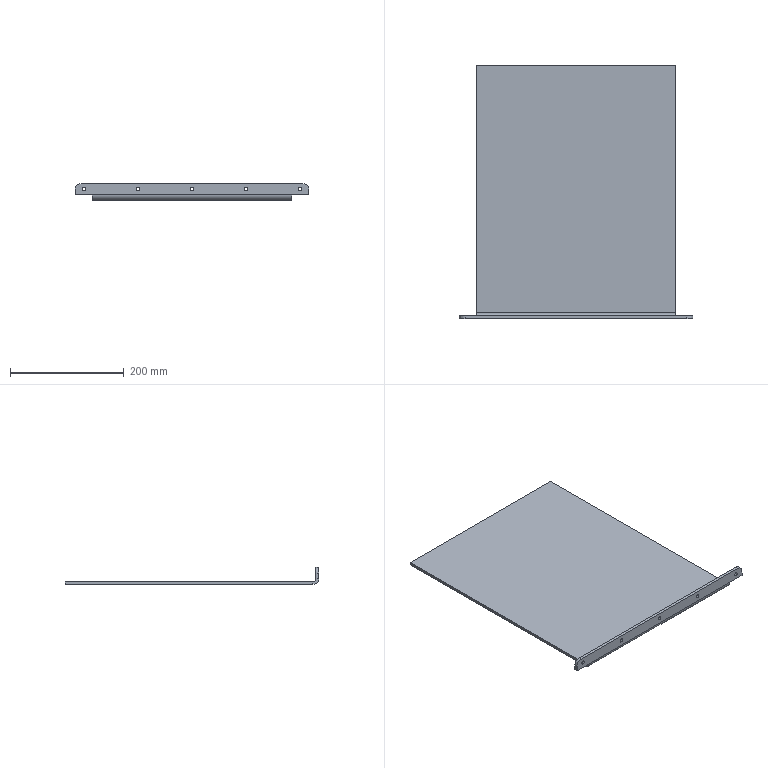Part | SolidWorks | features EdgeFlange 1, Fillet 1, FlatPattern 1, HoleWzd 1, LPattern 1, SMBaseFlange 1, SheetMetal 1 | 1 solid | 38 faces | box 410 x 445 x 30 mm | volume 821945 mm3 | cylinder 14 | plane 14 | cone 10 | commonest cylinder face diameters 6 x10 20 x3 10 x1
STEP:
#1=CARTESIAN_POINT('',(-95.,-222.475,23.));
#2=VERTEX_POINT('',#1);
#3=CARTESIAN_POINT('',(-95.,-222.475,17.));
#4=VERTEX_POINT('',#3);
#5=CARTESIAN_POINT('',(-95.,-222.475,20.));
#6=DIRECTION('',(0.,-1.,0.));
#7=DIRECTION('',(0.,0.,-1.));
#8=AXIS2_PLACEMENT_3D('',#5,#6,#7);
#9=CIRCLE('',#8,3.);
#10=EDGE_CURVE('',#2,#4,#9,.T.);
#11=ORIENTED_EDGE('',*,*,#10,.F.);
#12=CARTESIAN_POINT('',(-95.,-222.5,23.025));
#13=VERTEX_POINT('',#12);
#14=CARTESIAN_POINT('',(-95.,-222.5,23.025));
#15=DIRECTION('',(0.,-0.7071,0.7071));
#16=VECTOR('',#15,1000.);
#17=LINE('',#14,#16);
#18=EDGE_CURVE('',#2,#13,#17,.T.);
#19=ORIENTED_EDGE('',*,*,#18,.T.);
#20=CARTESIAN_POINT('',(-95.,-222.5,16.975));
#21=VERTEX_POINT('',#20);
#22=CARTESIAN_POINT('',(-95.,-222.5,20.));
#23=DIRECTION('',(0.,-1.,0.));
#24=DIRECTION('',(0.,0.,-1.));
#25=AXIS2_PLACEMENT_3D('',#22,#23,#24);
#26=CIRCLE('',#25,3.025);
#27=EDGE_CURVE('',#13,#21,#26,.T.);
#28=ORIENTED_EDGE('',*,*,#27,.T.);
#29=CARTESIAN_POINT('',(-95.,-222.5,16.975));
#30=DIRECTION('',(0.,-0.7071,-0.7071));
#31=VECTOR('',#30,1000.);
#32=LINE('',#29,#31);
#33=EDGE_CURVE('',#4,#21,#32,.T.);
#34=ORIENTED_EDGE('',*,*,#33,.F.);
#35=EDGE_LOOP('',(#11,#19,#28,#34));
#36=FACE_OUTER_BOUND('',#35,.T.);
#37=CARTESIAN_POINT('',(-95.,-222.5,20.));
#38=DIRECTION('',(0.,-1.,0.));
#39=DIRECTION('',(0.,0.,-1.));
#40=AXIS2_PLACEMENT_3D('',#37,#38,#39);
#41=CONICAL_SURFACE('',#40,3.025,0.7854);
#42=ADVANCED_FACE('',(#36),#41,.F.);
#43=CARTESIAN_POINT('',(-95.,-217.5,23.));
#44=VERTEX_POINT('',#43);
#45=CARTESIAN_POINT('',(-95.,-217.5,17.));
#46=VERTEX_POINT('',#45);
#47=CARTESIAN_POINT('',(-95.,-217.5,20.));
#48=DIRECTION('',(0.,-1.,0.));
#49=DIRECTION('',(0.,0.,-1.));
#50=AXIS2_PLACEMENT_3D('',#47,#48,#49);
#51=CIRCLE('',#50,3.);
#52=EDGE_CURVE('',#44,#46,#51,.T.);
#53=ORIENTED_EDGE('',*,*,#52,.F.);
#54=CARTESIAN_POINT('',(-95.,-222.5,23.));
#55=DIRECTION('',(0.,-1.,0.));
#56=VECTOR('',#55,1000.);
#57=LINE('',#54,#56);
#58=EDGE_CURVE('',#44,#2,#57,.T.);
#59=ORIENTED_EDGE('',*,*,#58,.T.);
#60=ORIENTED_EDGE('',*,*,#10,.T.);
#61=CARTESIAN_POINT('',(-95.,-222.5,17.));
#62=DIRECTION('',(0.,-1.,0.));
#63=VECTOR('',#62,1000.);
#64=LINE('',#61,#63);
#65=EDGE_CURVE('',#46,#4,#64,.T.);
#66=ORIENTED_EDGE('',*,*,#65,.F.);
#67=EDGE_LOOP('',(#53,#59,#60,#66));
#68=FACE_OUTER_BOUND('',#67,.T.);
#69=CARTESIAN_POINT('',(-95.,-222.5,20.));
#70=DIRECTION('',(0.,-1.,0.));
#71=DIRECTION('',(0.,0.,-1.));
#72=AXIS2_PLACEMENT_3D('',#69,#70,#71);
#73=CYLINDRICAL_SURFACE('',#72,3.);
#74=ADVANCED_FACE('',(#68),#73,.F.);
#75=CARTESIAN_POINT('',(-190.,-222.475,23.));
#76=VERTEX_POINT('',#75);
#77=CARTESIAN_POINT('',(-190.,-222.475,17.));
#78=VERTEX_POINT('',#77);
#79=CARTESIAN_POINT('',(-190.,-222.475,20.));
#80=DIRECTION('',(0.,-1.,0.));
#81=DIRECTION('',(0.,0.,-1.));
#82=AXIS2_PLACEMENT_3D('',#79,#80,#81);
#83=CIRCLE('',#82,3.);
#84=EDGE_CURVE('',#76,#78,#83,.T.);
#85=ORIENTED_EDGE('',*,*,#84,.F.);
#86=CARTESIAN_POINT('',(-190.,-222.5,23.025));
#87=VERTEX_POINT('',#86);
#88=CARTESIAN_POINT('',(-190.,-222.5,23.025));
#89=DIRECTION('',(0.,-0.7071,0.7071));
#90=VECTOR('',#89,1000.);
#91=LINE('',#88,#90);
#92=EDGE_CURVE('',#76,#87,#91,.T.);
#93=ORIENTED_EDGE('',*,*,#92,.T.);
#94=CARTESIAN_POINT('',(-190.,-222.5,16.975));
#95=VERTEX_POINT('',#94);
#96=CARTESIAN_POINT('',(-190.,-222.5,20.));
#97=DIRECTION('',(0.,-1.,0.));
#98=DIRECTION('',(0.,0.,-1.));
#99=AXIS2_PLACEMENT_3D('',#96,#97,#98);
#100=CIRCLE('',#99,3.025);
#101=EDGE_CURVE('',#87,#95,#100,.T.);
#102=ORIENTED_EDGE('',*,*,#101,.T.);
#103=CARTESIAN_POINT('',(-190.,-222.5,16.975));
#104=DIRECTION('',(0.,-0.7071,-0.7071));
#105=VECTOR('',#104,1000.);
#106=LINE('',#103,#105);
#107=EDGE_CURVE('',#78,#95,#106,.T.);
#108=ORIENTED_EDGE('',*,*,#107,.F.);
#109=EDGE_LOOP('',(#85,#93,#102,#108));
#110=FACE_OUTER_BOUND('',#109,.T.);
#111=CARTESIAN_POINT('',(-190.,-222.5,20.));
#112=DIRECTION('',(0.,-1.,0.));
#113=DIRECTION('',(0.,0.,-1.));
#114=AXIS2_PLACEMENT_3D('',#111,#112,#113);
#115=CONICAL_SURFACE('',#114,3.025,0.7854);
#116=ADVANCED_FACE('',(#110),#115,.F.);
#117=CARTESIAN_POINT('',(-190.,-217.5,23.));
#118=VERTEX_POINT('',#117);
#119=CARTESIAN_POINT('',(-190.,-217.5,17.));
#120=VERTEX_POINT('',#119);
#121=CARTESIAN_POINT('',(-190.,-217.5,20.));
#122=DIRECTION('',(0.,-1.,0.));
#123=DIRECTION('',(0.,0.,-1.));
#124=AXIS2_PLACEMENT_3D('',#121,#122,#123);
#125=CIRCLE('',#124,3.);
#126=EDGE_CURVE('',#118,#120,#125,.T.);
#127=ORIENTED_EDGE('',*,*,#126,.F.);
#128=CARTESIAN_POINT('',(-190.,-222.5,23.));
#129=DIRECTION('',(0.,-1.,0.));
#130=VECTOR('',#129,1000.);
#131=LINE('',#128,#130);
#132=EDGE_CURVE('',#118,#76,#131,.T.);
#133=ORIENTED_EDGE('',*,*,#132,.T.);
#134=ORIENTED_EDGE('',*,*,#84,.T.);
#135=CARTESIAN_POINT('',(-190.,-222.5,17.));
#136=DIRECTION('',(0.,-1.,0.));
#137=VECTOR('',#136,1000.);
#138=LINE('',#135,#137);
#139=EDGE_CURVE('',#120,#78,#138,.T.);
#140=ORIENTED_EDGE('',*,*,#139,.F.);
#141=EDGE_LOOP('',(#127,#133,#134,#140));
#142=FACE_OUTER_BOUND('',#141,.T.);
#143=CARTESIAN_POINT('',(-190.,-222.5,20.));
#144=DIRECTION('',(0.,-1.,0.));
#145=DIRECTION('',(0.,0.,-1.));
#146=AXIS2_PLACEMENT_3D('',#143,#144,#145);
#147=CYLINDRICAL_SURFACE('',#146,3.);
#148=ADVANCED_FACE('',(#142),#147,.F.);
#149=CARTESIAN_POINT('',(0.,-217.5,23.));
#150=VERTEX_POINT('',#149);
#151=CARTESIAN_POINT('',(0.,-217.5,17.));
#152=VERTEX_POINT('',#151);
#153=CARTESIAN_POINT('',(0.,-217.5,20.));
#154=DIRECTION('',(0.,-1.,0.));
#155=DIRECTION('',(0.,0.,-1.));
#156=AXIS2_PLACEMENT_3D('',#153,#154,#155);
#157=CIRCLE('',#156,3.);
#158=EDGE_CURVE('',#150,#152,#157,.T.);
#159=ORIENTED_EDGE('',*,*,#158,.F.);
#160=CARTESIAN_POINT('',(0.,-222.475,23.));
#161=VERTEX_POINT('',#160);
#162=CARTESIAN_POINT('',(0.,-222.5,23.));
#163=DIRECTION('',(0.,-1.,0.));
#164=VECTOR('',#163,1000.);
#165=LINE('',#162,#164);
#166=EDGE_CURVE('',#150,#161,#165,.T.);
#167=ORIENTED_EDGE('',*,*,#166,.T.);
#168=CARTESIAN_POINT('',(0.,-222.475,17.));
#169=VERTEX_POINT('',#168);
#170=CARTESIAN_POINT('',(0.,-222.475,20.));
#171=DIRECTION('',(0.,-1.,0.));
#172=DIRECTION('',(0.,0.,-1.));
#173=AXIS2_PLACEMENT_3D('',#170,#171,#172);
#174=CIRCLE('',#173,3.);
#175=EDGE_CURVE('',#161,#169,#174,.T.);
#176=ORIENTED_EDGE('',*,*,#175,.T.);
#177=CARTESIAN_POINT('',(0.,-222.5,17.));
#178=DIRECTION('',(0.,-1.,0.));
#179=VECTOR('',#178,1000.);
#180=LINE('',#177,#179);
#181=EDGE_CURVE('',#152,#169,#180,.T.);
#182=ORIENTED_EDGE('',*,*,#181,.F.);
#183=EDGE_LOOP('',(#159,#167,#176,#182));
#184=FACE_OUTER_BOUND('',#183,.T.);
#185=CARTESIAN_POINT('',(0.,-222.5,20.));
#186=DIRECTION('',(0.,-1.,0.));
#187=DIRECTION('',(0.,0.,-1.));
#188=AXIS2_PLACEMENT_3D('',#185,#186,#187);
#189=CYLINDRICAL_SURFACE('',#188,3.);
#190=ADVANCED_FACE('',(#184),#189,.F.);
#191=ORIENTED_EDGE('',*,*,#175,.F.);
#192=CARTESIAN_POINT('',(0.,-222.5,23.025));
#193=VERTEX_POINT('',#192);
#194=CARTESIAN_POINT('',(0.,-222.5,23.025));
#195=DIRECTION('',(0.,-0.7071,0.7071));
#196=VECTOR('',#195,1000.);
#197=LINE('',#194,#196);
#198=EDGE_CURVE('',#161,#193,#197,.T.);
#199=ORIENTED_EDGE('',*,*,#198,.T.);
#200=CARTESIAN_POINT('',(0.,-222.5,16.975));
#201=VERTEX_POINT('',#200);
#202=CARTESIAN_POINT('',(0.,-222.5,20.));
#203=DIRECTION('',(0.,-1.,0.));
#204=DIRECTION('',(0.,0.,-1.));
#205=AXIS2_PLACEMENT_3D('',#202,#203,#204);
#206=CIRCLE('',#205,3.025);
#207=EDGE_CURVE('',#193,#201,#206,.T.);
#208=ORIENTED_EDGE('',*,*,#207,.T.);
#209=CARTESIAN_POINT('',(0.,-222.5,16.975));
#210=DIRECTION('',(0.,-0.7071,-0.7071));
#211=VECTOR('',#210,1000.);
#212=LINE('',#209,#211);
#213=EDGE_CURVE('',#169,#201,#212,.T.);
#214=ORIENTED_EDGE('',*,*,#213,.F.);
#215=EDGE_LOOP('',(#191,#199,#208,#214));
#216=FACE_OUTER_BOUND('',#215,.T.);
#217=CARTESIAN_POINT('',(0.,-222.5,20.));
#218=DIRECTION('',(0.,-1.,0.));
#219=DIRECTION('',(0.,0.,-1.));
#220=AXIS2_PLACEMENT_3D('',#217,#218,#219);
#221=CONICAL_SURFACE('',#220,3.025,0.7854);
#222=ADVANCED_FACE('',(#216),#221,.F.);
#223=CARTESIAN_POINT('',(95.,-217.5,23.));
#224=VERTEX_POINT('',#223);
#225=CARTESIAN_POINT('',(95.,-217.5,17.));
#226=VERTEX_POINT('',#225);
#227=CARTESIAN_POINT('',(95.,-217.5,20.));
#228=DIRECTION('',(0.,-1.,0.));
#229=DIRECTION('',(0.,0.,-1.));
#230=AXIS2_PLACEMENT_3D('',#227,#228,#229);
#231=CIRCLE('',#230,3.);
#232=EDGE_CURVE('',#224,#226,#231,.T.);
#233=ORIENTED_EDGE('',*,*,#232,.F.);
#234=CARTESIAN_POINT('',(95.,-222.475,23.));
#235=VERTEX_POINT('',#234);
#236=CARTESIAN_POINT('',(95.,-222.5,23.));
#237=DIRECTION('',(0.,-1.,0.));
#238=VECTOR('',#237,1000.);
#239=LINE('',#236,#238);
#240=EDGE_CURVE('',#224,#235,#239,.T.);
#241=ORIENTED_EDGE('',*,*,#240,.T.);
#242=CARTESIAN_POINT('',(95.,-222.475,17.));
#243=VERTEX_POINT('',#242);
#244=CARTESIAN_POINT('',(95.,-222.475,20.));
#245=DIRECTION('',(0.,-1.,0.));
#246=DIRECTION('',(0.,0.,-1.));
#247=AXIS2_PLACEMENT_3D('',#244,#245,#246);
#248=CIRCLE('',#247,3.);
#249=EDGE_CURVE('',#235,#243,#248,.T.);
#250=ORIENTED_EDGE('',*,*,#249,.T.);
#251=CARTESIAN_POINT('',(95.,-222.5,17.));
#252=DIRECTION('',(0.,-1.,0.));
#253=VECTOR('',#252,1000.);
#254=LINE('',#251,#253);
#255=EDGE_CURVE('',#226,#243,#254,.T.);
#256=ORIENTED_EDGE('',*,*,#255,.F.);
#257=EDGE_LOOP('',(#233,#241,#250,#256));
#258=FACE_OUTER_BOUND('',#257,.T.);
#259=CARTESIAN_POINT('',(95.,-222.5,20.));
#260=DIRECTION('',(0.,-1.,0.));
#261=DIRECTION('',(0.,0.,-1.));
#262=AXIS2_PLACEMENT_3D('',#259,#260,#261);
#263=CYLINDRICAL_SURFACE('',#262,3.);
#264=ADVANCED_FACE('',(#258),#263,.F.);
#265=ORIENTED_EDGE('',*,*,#249,.F.);
#266=CARTESIAN_POINT('',(95.,-222.5,23.025));
#267=VERTEX_POINT('',#266);
#268=CARTESIAN_POINT('',(95.,-222.5,23.025));
#269=DIRECTION('',(0.,-0.7071,0.7071));
#270=VECTOR('',#269,1000.);
#271=LINE('',#268,#270);
#272=EDGE_CURVE('',#235,#267,#271,.T.);
#273=ORIENTED_EDGE('',*,*,#272,.T.);
#274=CARTESIAN_POINT('',(95.,-222.5,16.975));
#275=VERTEX_POINT('',#274);
#276=CARTESIAN_POINT('',(95.,-222.5,20.));
#277=DIRECTION('',(0.,-1.,0.));
#278=DIRECTION('',(0.,0.,-1.));
#279=AXIS2_PLACEMENT_3D('',#276,#277,#278);
#280=CIRCLE('',#279,3.025);
#281=EDGE_CURVE('',#267,#275,#280,.T.);
#282=ORIENTED_EDGE('',*,*,#281,.T.);
#283=CARTESIAN_POINT('',(95.,-222.5,16.975));
#284=DIRECTION('',(0.,-0.7071,-0.7071));
#285=VECTOR('',#284,1000.);
#286=LINE('',#283,#285);
#287=EDGE_CURVE('',#243,#275,#286,.T.);
#288=ORIENTED_EDGE('',*,*,#287,.F.);
#289=EDGE_LOOP('',(#265,#273,#282,#288));
#290=FACE_OUTER_BOUND('',#289,.T.);
#291=CARTESIAN_POINT('',(95.,-222.5,20.));
#292=DIRECTION('',(0.,-1.,0.));
#293=DIRECTION('',(0.,0.,-1.));
#294=AXIS2_PLACEMENT_3D('',#291,#292,#293);
#295=CONICAL_SURFACE('',#294,3.025,0.7854);
#296=ADVANCED_FACE('',(#290),#295,.F.);
#297=CARTESIAN_POINT('',(190.,-217.5,23.));
#298=VERTEX_POINT('',#297);
#299=CARTESIAN_POINT('',(190.,-217.5,17.));
#300=VERTEX_POINT('',#299);
#301=CARTESIAN_POINT('',(190.,-217.5,20.));
#302=DIRECTION('',(0.,-1.,0.));
#303=DIRECTION('',(0.,0.,-1.));
#304=AXIS2_PLACEMENT_3D('',#301,#302,#303);
#305=CIRCLE('',#304,3.);
#306=EDGE_CURVE('',#298,#300,#305,.T.);
#307=ORIENTED_EDGE('',*,*,#306,.F.);
#308=CARTESIAN_POINT('',(190.,-222.475,23.));
#309=VERTEX_POINT('',#308);
#310=CARTESIAN_POINT('',(190.,-222.5,23.));
#311=DIRECTION('',(0.,-1.,0.));
#312=VECTOR('',#311,1000.);
#313=LINE('',#310,#312);
#314=EDGE_CURVE('',#298,#309,#313,.T.);
#315=ORIENTED_EDGE('',*,*,#314,.T.);
#316=CARTESIAN_POINT('',(190.,-222.475,17.));
#317=VERTEX_POINT('',#316);
#318=CARTESIAN_POINT('',(190.,-222.475,20.));
#319=DIRECTION('',(0.,-1.,0.));
#320=DIRECTION('',(0.,0.,-1.));
#321=AXIS2_PLACEMENT_3D('',#318,#319,#320);
#322=CIRCLE('',#321,3.);
#323=EDGE_CURVE('',#309,#317,#322,.T.);
#324=ORIENTED_EDGE('',*,*,#323,.T.);
#325=CARTESIAN_POINT('',(190.,-222.5,17.));
#326=DIRECTION('',(0.,-1.,0.));
#327=VECTOR('',#326,1000.);
#328=LINE('',#325,#327);
#329=EDGE_CURVE('',#300,#317,#328,.T.);
#330=ORIENTED_EDGE('',*,*,#329,.F.);
#331=EDGE_LOOP('',(#307,#315,#324,#330));
#332=FACE_OUTER_BOUND('',#331,.T.);
#333=CARTESIAN_POINT('',(190.,-222.5,20.));
#334=DIRECTION('',(0.,-1.,0.));
#335=DIRECTION('',(0.,0.,-1.));
#336=AXIS2_PLACEMENT_3D('',#333,#334,#335);
#337=CYLINDRICAL_SURFACE('',#336,3.);
#338=ADVANCED_FACE('',(#332),#337,.F.);
#339=ORIENTED_EDGE('',*,*,#323,.F.);
#340=CARTESIAN_POINT('',(190.,-222.5,23.025));
#341=VERTEX_POINT('',#340);
#342=CARTESIAN_POINT('',(190.,-222.5,23.025));
#343=DIRECTION('',(0.,-0.7071,0.7071));
#344=VECTOR('',#343,1000.);
#345=LINE('',#342,#344);
#346=EDGE_CURVE('',#309,#341,#345,.T.);
#347=ORIENTED_EDGE('',*,*,#346,.T.);
#348=CARTESIAN_POINT('',(190.,-222.5,16.975));
#349=VERTEX_POINT('',#348);
#350=CARTESIAN_POINT('',(190.,-222.5,20.));
#351=DIRECTION('',(0.,-1.,0.));
#352=DIRECTION('',(0.,0.,-1.));
#353=AXIS2_PLACEMENT_3D('',#350,#351,#352);
#354=CIRCLE('',#353,3.025);
#355=EDGE_CURVE('',#341,#349,#354,.T.);
#356=ORIENTED_EDGE('',*,*,#355,.T.);
#357=CARTESIAN_POINT('',(190.,-222.5,16.975));
#358=DIRECTION('',(0.,-0.7071,-0.7071));
#359=VECTOR('',#358,1000.);
#360=LINE('',#357,#359);
#361=EDGE_CURVE('',#317,#349,#360,.T.);
#362=ORIENTED_EDGE('',*,*,#361,.F.);
#363=EDGE_LOOP('',(#339,#347,#356,#362));
#364=FACE_OUTER_BOUND('',#363,.T.);
#365=CARTESIAN_POINT('',(190.,-222.5,20.));
#366=DIRECTION('',(0.,-1.,0.));
#367=DIRECTION('',(0.,0.,-1.));
#368=AXIS2_PLACEMENT_3D('',#365,#366,#367);
#369=CONICAL_SURFACE('',#368,3.025,0.7854);
#370=ADVANCED_FACE('',(#364),#369,.F.);
#371=ORIENTED_EDGE('',*,*,#346,.F.);
#372=CARTESIAN_POINT('',(190.,-222.475,20.));
#373=DIRECTION('',(0.,-1.,0.));
#374=DIRECTION('',(0.,0.,-1.));
#375=AXIS2_PLACEMENT_3D('',#372,#373,#374);
#376=CIRCLE('',#375,3.);
#377=EDGE_CURVE('',#317,#309,#376,.T.);
#378=ORIENTED_EDGE('',*,*,#377,.F.);
#379=ORIENTED_EDGE('',*,*,#361,.T.);
#380=CARTESIAN_POINT('',(190.,-222.5,20.));
#381=DIRECTION('',(0.,-1.,0.));
#382=DIRECTION('',(0.,0.,-1.));
#383=AXIS2_PLACEMENT_3D('',#380,#381,#382);
#384=CIRCLE('',#383,3.025);
#385=EDGE_CURVE('',#349,#341,#384,.T.);
#386=ORIENTED_EDGE('',*,*,#385,.T.);
#387=EDGE_LOOP('',(#371,#378,#379,#386));
#388=FACE_OUTER_BOUND('',#387,.T.);
#389=CARTESIAN_POINT('',(190.,-222.5,20.));
#390=DIRECTION('',(0.,-1.,0.));
#391=DIRECTION('',(0.,0.,-1.));
#392=AXIS2_PLACEMENT_3D('',#389,#390,#391);
#393=CONICAL_SURFACE('',#392,3.025,0.7854);
#394=ADVANCED_FACE('',(#388),#393,.F.);
#395=ORIENTED_EDGE('',*,*,#314,.F.);
#396=CARTESIAN_POINT('',(190.,-217.5,20.));
#397=DIRECTION('',(0.,-1.,0.));
#398=DIRECTION('',(0.,0.,-1.));
#399=AXIS2_PLACEMENT_3D('',#396,#397,#398);
#400=CIRCLE('',#399,3.);
#401=EDGE_CURVE('',#300,#298,#400,.T.);
#402=ORIENTED_EDGE('',*,*,#401,.F.);
#403=ORIENTED_EDGE('',*,*,#329,.T.);
#404=ORIENTED_EDGE('',*,*,#377,.T.);
#405=EDGE_LOOP('',(#395,#402,#403,#404));
#406=FACE_OUTER_BOUND('',#405,.T.);
#407=CARTESIAN_POINT('',(190.,-222.5,20.));
#408=DIRECTION('',(0.,-1.,0.));
#409=DIRECTION('',(0.,0.,-1.));
#410=AXIS2_PLACEMENT_3D('',#407,#408,#409);
#411=CYLINDRICAL_SURFACE('',#410,3.);
#412=ADVANCED_FACE('',(#406),#411,.F.);
#413=ORIENTED_EDGE('',*,*,#272,.F.);
#414=CARTESIAN_POINT('',(95.,-222.475,20.));
#415=DIRECTION('',(0.,-1.,0.));
#416=DIRECTION('',(0.,0.,-1.));
#417=AXIS2_PLACEMENT_3D('',#414,#415,#416);
#418=CIRCLE('',#417,3.);
#419=EDGE_CURVE('',#243,#235,#418,.T.);
#420=ORIENTED_EDGE('',*,*,#419,.F.);
#421=ORIENTED_EDGE('',*,*,#287,.T.);
#422=CARTESIAN_POINT('',(95.,-222.5,20.));
#423=DIRECTION('',(0.,-1.,0.));
#424=DIRECTION('',(0.,0.,-1.));
#425=AXIS2_PLACEMENT_3D('',#422,#423,#424);
#426=CIRCLE('',#425,3.025);
#427=EDGE_CURVE('',#275,#267,#426,.T.);
#428=ORIENTED_EDGE('',*,*,#427,.T.);
#429=EDGE_LOOP('',(#413,#420,#421,#428));
#430=FACE_OUTER_BOUND('',#429,.T.);
#431=CARTESIAN_POINT('',(95.,-222.5,20.));
#432=DIRECTION('',(0.,-1.,0.));
#433=DIRECTION('',(0.,0.,-1.));
#434=AXIS2_PLACEMENT_3D('',#431,#432,#433);
#435=CONICAL_SURFACE('',#434,3.025,0.7854);
#436=ADVANCED_FACE('',(#430),#435,.F.);
#437=ORIENTED_EDGE('',*,*,#240,.F.);
#438=CARTESIAN_POINT('',(95.,-217.5,20.));
#439=DIRECTION('',(0.,-1.,0.));
#440=DIRECTION('',(0.,0.,-1.));
#441=AXIS2_PLACEMENT_3D('',#438,#439,#440);
#442=CIRCLE('',#441,3.);
#443=EDGE_CURVE('',#226,#224,#442,.T.);
#444=ORIENTED_EDGE('',*,*,#443,.F.);
#445=ORIENTED_EDGE('',*,*,#255,.T.);
#446=ORIENTED_EDGE('',*,*,#419,.T.);
#447=EDGE_LOOP('',(#437,#444,#445,#446));
#448=FACE_OUTER_BOUND('',#447,.T.);
#449=CARTESIAN_POINT('',(95.,-222.5,20.));
#450=DIRECTION('',(0.,-1.,0.));
#451=DIRECTION('',(0.,0.,-1.));
#452=AXIS2_PLACEMENT_3D('',#449,#450,#451);
#453=CYLINDRICAL_SURFACE('',#452,3.);
#454=ADVANCED_FACE('',(#448),#453,.F.);
#455=ORIENTED_EDGE('',*,*,#198,.F.);
#456=CARTESIAN_POINT('',(0.,-222.475,20.));
#457=DIRECTION('',(0.,-1.,0.));
#458=DIRECTION('',(0.,0.,-1.));
#459=AXIS2_PLACEMENT_3D('',#456,#457,#458);
#460=CIRCLE('',#459,3.);
#461=EDGE_CURVE('',#169,#161,#460,.T.);
#462=ORIENTED_EDGE('',*,*,#461,.F.);
#463=ORIENTED_EDGE('',*,*,#213,.T.);
#464=CARTESIAN_POINT('',(0.,-222.5,20.));
#465=DIRECTION('',(0.,-1.,0.));
#466=DIRECTION('',(0.,0.,-1.));
#467=AXIS2_PLACEMENT_3D('',#464,#465,#466);
#468=CIRCLE('',#467,3.025);
#469=EDGE_CURVE('',#201,#193,#468,.T.);
#470=ORIENTED_EDGE('',*,*,#469,.T.);
#471=EDGE_LOOP('',(#455,#462,#463,#470));
#472=FACE_OUTER_BOUND('',#471,.T.);
#473=CARTESIAN_POINT('',(0.,-222.5,20.));
#474=DIRECTION('',(0.,-1.,0.));
#475=DIRECTION('',(0.,0.,-1.));
#476=AXIS2_PLACEMENT_3D('',#473,#474,#475);
#477=CONICAL_SURFACE('',#476,3.025,0.7854);
#478=ADVANCED_FACE('',(#472),#477,.F.);
#479=ORIENTED_EDGE('',*,*,#166,.F.);
#480=CARTESIAN_POINT('',(0.,-217.5,20.));
#481=DIRECTION('',(0.,-1.,0.));
#482=DIRECTION('',(0.,0.,-1.));
#483=AXIS2_PLACEMENT_3D('',#480,#481,#482);
#484=CIRCLE('',#483,3.);
#485=EDGE_CURVE('',#152,#150,#484,.T.);
#486=ORIENTED_EDGE('',*,*,#485,.F.);
#487=ORIENTED_EDGE('',*,*,#181,.T.);
#488=ORIENTED_EDGE('',*,*,#461,.T.);
#489=EDGE_LOOP('',(#479,#486,#487,#488));
#490=FACE_OUTER_BOUND('',#489,.T.);
#491=CARTESIAN_POINT('',(0.,-222.5,20.));
#492=DIRECTION('',(0.,-1.,0.));
#493=DIRECTION('',(0.,0.,-1.));
#494=AXIS2_PLACEMENT_3D('',#491,#492,#493);
#495=CYLINDRICAL_SURFACE('',#494,3.);
#496=ADVANCED_FACE('',(#490),#495,.F.);
#497=CARTESIAN_POINT('',(175.,-212.5,5.));
#498=VERTEX_POINT('',#497);
#499=CARTESIAN_POINT('',(175.,-212.5,0.));
#500=VERTEX_POINT('',#499);
#501=CARTESIAN_POINT('',(175.,-212.5,5.));
#502=DIRECTION('',(0.,0.,-1.));
#503=VECTOR('',#502,1000.);
#504=LINE('',#501,#503);
#505=EDGE_CURVE('',#498,#500,#504,.T.);
#506=ORIENTED_EDGE('',*,*,#505,.T.);
#507=CARTESIAN_POINT('',(175.,222.5,0.));
#508=VERTEX_POINT('',#507);
#509=CARTESIAN_POINT('',(175.,222.5,0.));
#510=DIRECTION('',(0.,1.,0.));
#511=VECTOR('',#510,1000.);
#512=LINE('',#509,#511);
#513=EDGE_CURVE('',#500,#508,#512,.T.);
#514=ORIENTED_EDGE('',*,*,#513,.T.);
#515=CARTESIAN_POINT('',(175.,222.5,5.));
#516=VERTEX_POINT('',#515);
#517=CARTESIAN_POINT('',(175.,222.5,5.));
#518=DIRECTION('',(0.,0.,-1.));
#519=VECTOR('',#518,1000.);
#520=LINE('',#517,#519);
#521=EDGE_CURVE('',#516,#508,#520,.T.);
#522=ORIENTED_EDGE('',*,*,#521,.F.);
#523=CARTESIAN_POINT('',(175.,222.5,5.));
#524=DIRECTION('',(0.,1.,0.));
#525=VECTOR('',#524,1000.);
#526=LINE('',#523,#525);
#527=EDGE_CURVE('',#498,#516,#526,.T.);
#528=ORIENTED_EDGE('',*,*,#527,.F.);
#529=EDGE_LOOP('',(#506,#514,#522,#528));
#530=FACE_OUTER_BOUND('',#529,.T.);
#531=CARTESIAN_POINT('',(175.,222.5,5.));
#532=DIRECTION('',(-1.,0.,0.));
#533=DIRECTION('',(0.,-1.,0.));
#534=AXIS2_PLACEMENT_3D('',#531,#532,#533);
#535=PLANE('',#534);
#536=ADVANCED_FACE('',(#530),#535,.F.);
#537=CARTESIAN_POINT('',(-175.,-212.5,5.));
#538=VERTEX_POINT('',#537);
#539=CARTESIAN_POINT('',(-175.,-212.5,0.));
#540=VERTEX_POINT('',#539);
#541=CARTESIAN_POINT('',(-175.,-212.5,5.));
#542=DIRECTION('',(0.,0.,-1.));
#543=VECTOR('',#542,1000.);
#544=LINE('',#541,#543);
#545=EDGE_CURVE('',#538,#540,#544,.T.);
#546=ORIENTED_EDGE('',*,*,#545,.F.);
#547=CARTESIAN_POINT('',(-175.,222.5,5.));
#548=VERTEX_POINT('',#547);
#549=CARTESIAN_POINT('',(-175.,222.5,5.));
#550=DIRECTION('',(0.,-1.,0.));
#551=VECTOR('',#550,1000.);
#552=LINE('',#549,#551);
#553=EDGE_CURVE('',#548,#538,#552,.T.);
#554=ORIENTED_EDGE('',*,*,#553,.F.);
#555=CARTESIAN_POINT('',(-175.,222.5,0.));
#556=VERTEX_POINT('',#555);
#557=CARTESIAN_POINT('',(-175.,222.5,5.));
#558=DIRECTION('',(0.,0.,-1.));
#559=VECTOR('',#558,1000.);
#560=LINE('',#557,#559);
#561=EDGE_CURVE('',#548,#556,#560,.T.);
#562=ORIENTED_EDGE('',*,*,#561,.T.);
#563=CARTESIAN_POINT('',(-175.,222.5,0.));
#564=DIRECTION('',(0.,-1.,0.));
#565=VECTOR('',#564,1000.);
#566=LINE('',#563,#565);
#567=EDGE_CURVE('',#556,#540,#566,.T.);
#568=ORIENTED_EDGE('',*,*,#567,.T.);
#569=EDGE_LOOP('',(#546,#554,#562,#568));
#570=FACE_OUTER_BOUND('',#569,.T.);
#571=CARTESIAN_POINT('',(-175.,222.5,5.));
#572=DIRECTION('',(1.,0.,0.));
#573=DIRECTION('',(0.,1.,0.));
#574=AXIS2_PLACEMENT_3D('',#571,#572,#573);
#575=PLANE('',#574);
#576=ADVANCED_FACE('',(#570),#575,.F.);
#577=ORIENTED_EDGE('',*,*,#553,.T.);
#578=CARTESIAN_POINT('',(175.,-212.5,5.));
#579=DIRECTION('',(-1.,0.,0.));
#580=VECTOR('',#579,1000.);
#581=LINE('',#578,#580);
#582=EDGE_CURVE('',#498,#538,#581,.T.);
#583=ORIENTED_EDGE('',*,*,#582,.F.);
#584=ORIENTED_EDGE('',*,*,#527,.T.);
#585=CARTESIAN_POINT('',(-175.,222.5,5.));
#586=DIRECTION('',(-1.,0.,0.));
#587=VECTOR('',#586,1000.);
#588=LINE('',#585,#587);
#589=EDGE_CURVE('',#516,#548,#588,.T.);
#590=ORIENTED_EDGE('',*,*,#589,.T.);
#591=EDGE_LOOP('',(#577,#583,#584,#590));
#592=FACE_OUTER_BOUND('',#591,.T.);
#593=CARTESIAN_POINT('',(0.,0.,5.));
#594=DIRECTION('',(0.,0.,1.));
#595=DIRECTION('',(1.,0.,0.));
#596=AXIS2_PLACEMENT_3D('',#593,#594,#595);
#597=PLANE('',#596);
#598=ADVANCED_FACE('',(#592),#597,.T.);
#599=CARTESIAN_POINT('',(175.,-212.5,0.));
#600=DIRECTION('',(-1.,0.,0.));
#601=VECTOR('',#600,1000.);
#602=LINE('',#599,#601);
#603=EDGE_CURVE('',#500,#540,#602,.T.);
#604=ORIENTED_EDGE('',*,*,#603,.T.);
#605=ORIENTED_EDGE('',*,*,#567,.F.);
#606=CARTESIAN_POINT('',(-175.,222.5,0.));
#607=DIRECTION('',(-1.,0.,0.));
#608=VECTOR('',#607,1000.);
#609=LINE('',#606,#608);
#610=EDGE_CURVE('',#508,#556,#609,.T.);
#611=ORIENTED_EDGE('',*,*,#610,.F.);
#612=ORIENTED_EDGE('',*,*,#513,.F.);
#613=EDGE_LOOP('',(#604,#605,#611,#612));
#614=FACE_OUTER_BOUND('',#613,.T.);
#615=CARTESIAN_POINT('',(0.,0.,0.));
#616=DIRECTION('',(0.,0.,1.));
#617=DIRECTION('',(1.,0.,0.));
#618=AXIS2_PLACEMENT_3D('',#615,#616,#617);
#619=PLANE('',#618);
#620=ADVANCED_FACE('',(#614),#619,.F.);
#621=ORIENTED_EDGE('',*,*,#610,.T.);
#622=ORIENTED_EDGE('',*,*,#561,.F.);
#623=ORIENTED_EDGE('',*,*,#589,.F.);
#624=ORIENTED_EDGE('',*,*,#521,.T.);
#625=EDGE_LOOP('',(#621,#622,#623,#624));
#626=FACE_OUTER_BOUND('',#625,.T.);
#627=CARTESIAN_POINT('',(-175.,222.5,5.));
#628=DIRECTION('',(0.,-1.,0.));
#629=DIRECTION('',(0.,0.,-1.));
#630=AXIS2_PLACEMENT_3D('',#627,#628,#629);
#631=PLANE('',#630);
#632=ADVANCED_FACE('',(#626),#631,.F.);
#633=CARTESIAN_POINT('',(-175.,-217.5,10.));
#634=VERTEX_POINT('',#633);
#635=CARTESIAN_POINT('',(-175.,-222.5,10.));
#636=VERTEX_POINT('',#635);
#637=CARTESIAN_POINT('',(-175.,-217.5,10.));
#638=DIRECTION('',(0.,-1.,0.));
#639=VECTOR('',#638,1000.);
#640=LINE('',#637,#639);
#641=EDGE_CURVE('',#634,#636,#640,.T.);
#642=ORIENTED_EDGE('',*,*,#641,.F.);
#643=CARTESIAN_POINT('',(-175.,-212.5,10.));
#644=DIRECTION('',(-1.,0.,0.));
#645=DIRECTION('',(0.,0.,-1.));
#646=AXIS2_PLACEMENT_3D('',#643,#644,#645);
#647=CIRCLE('',#646,5.);
#648=EDGE_CURVE('',#538,#634,#647,.T.);
#649=ORIENTED_EDGE('',*,*,#648,.F.);
#650=ORIENTED_EDGE('',*,*,#545,.T.);
#651=CARTESIAN_POINT('',(-175.,-212.5,10.));
#652=DIRECTION('',(-1.,0.,0.));
#653=DIRECTION('',(0.,0.,-1.));
#654=AXIS2_PLACEMENT_3D('',#651,#652,#653);
#655=CIRCLE('',#654,10.);
#656=EDGE_CURVE('',#540,#636,#655,.T.);
#657=ORIENTED_EDGE('',*,*,#656,.T.);
#658=EDGE_LOOP('',(#642,#649,#650,#657));
#659=FACE_OUTER_BOUND('',#658,.T.);
#660=CARTESIAN_POINT('',(-175.,-212.5,10.));
#661=DIRECTION('',(-1.,0.,0.));
#662=DIRECTION('',(0.,0.,1.));
#663=AXIS2_PLACEMENT_3D('',#660,#661,#662);
#664=PLANE('',#663);
#665=ADVANCED_FACE('',(#659),#664,.T.);
#666=CARTESIAN_POINT('',(175.,-217.5,10.));
#667=VERTEX_POINT('',#666);
#668=CARTESIAN_POINT('',(175.,-212.5,10.));
#669=DIRECTION('',(1.,0.,0.));
#670=DIRECTION('',(0.,0.,-1.));
#671=AXIS2_PLACEMENT_3D('',#668,#669,#670);
#672=CIRCLE('',#671,5.);
#673=EDGE_CURVE('',#667,#498,#672,.T.);
#674=ORIENTED_EDGE('',*,*,#673,.F.);
#675=CARTESIAN_POINT('',(175.,-222.5,10.));
#676=VERTEX_POINT('',#675);
#677=CARTESIAN_POINT('',(175.,-217.5,10.));
#678=DIRECTION('',(0.,-1.,0.));
#679=VECTOR('',#678,1000.);
#680=LINE('',#677,#679);
#681=EDGE_CURVE('',#667,#676,#680,.T.);
#682=ORIENTED_EDGE('',*,*,#681,.T.);
#683=CARTESIAN_POINT('',(175.,-212.5,10.));
#684=DIRECTION('',(1.,0.,0.));
#685=DIRECTION('',(0.,0.,-1.));
#686=AXIS2_PLACEMENT_3D('',#683,#684,#685);
#687=CIRCLE('',#686,10.);
#688=EDGE_CURVE('',#676,#500,#687,.T.);
#689=ORIENTED_EDGE('',*,*,#688,.T.);
#690=ORIENTED_EDGE('',*,*,#505,.F.);
#691=EDGE_LOOP('',(#674,#682,#689,#690));
#692=FACE_OUTER_BOUND('',#691,.T.);
#693=CARTESIAN_POINT('',(175.,-212.5,10.));
#694=DIRECTION('',(-1.,0.,0.));
#695=DIRECTION('',(0.,0.,1.));
#696=AXIS2_PLACEMENT_3D('',#693,#694,#695);
#697=PLANE('',#696);
#698=ADVANCED_FACE('',(#692),#697,.F.);
#699=ORIENTED_EDGE('',*,*,#603,.F.);
#700=ORIENTED_EDGE('',*,*,#688,.F.);
#701=CARTESIAN_POINT('',(175.,-222.5,10.));
#702=DIRECTION('',(1.,0.,0.));
#703=VECTOR('',#702,1000.);
#704=LINE('',#701,#703);
#705=EDGE_CURVE('',#636,#676,#704,.T.);
#706=ORIENTED_EDGE('',*,*,#705,.F.);
#707=ORIENTED_EDGE('',*,*,#656,.F.);
#708=EDGE_LOOP('',(#699,#700,#706,#707));
#709=FACE_OUTER_BOUND('',#708,.T.);
#710=CARTESIAN_POINT('',(175.,-212.5,10.));
#711=DIRECTION('',(1.,0.,0.));
#712=DIRECTION('',(0.,-1.,0.));
#713=AXIS2_PLACEMENT_3D('',#710,#711,#712);
#714=CYLINDRICAL_SURFACE('',#713,10.);
#715=ADVANCED_FACE('',(#709),#714,.T.);
#716=ORIENTED_EDGE('',*,*,#582,.T.);
#717=ORIENTED_EDGE('',*,*,#648,.T.);
#718=CARTESIAN_POINT('',(175.,-217.5,10.));
#719=DIRECTION('',(1.,0.,0.));
#720=VECTOR('',#719,1000.);
#721=LINE('',#718,#720);
#722=EDGE_CURVE('',#634,#667,#721,.T.);
#723=ORIENTED_EDGE('',*,*,#722,.T.);
#724=ORIENTED_EDGE('',*,*,#673,.T.);
#725=EDGE_LOOP('',(#716,#717,#723,#724));
#726=FACE_OUTER_BOUND('',#725,.T.);
#727=CARTESIAN_POINT('',(175.,-212.5,10.));
#728=DIRECTION('',(1.,0.,0.));
#729=DIRECTION('',(0.,-1.,0.));
#730=AXIS2_PLACEMENT_3D('',#727,#728,#729);
#731=CYLINDRICAL_SURFACE('',#730,5.);
#732=ADVANCED_FACE('',(#726),#731,.F.);
#733=ORIENTED_EDGE('',*,*,#681,.F.);
#734=CARTESIAN_POINT('',(205.,-217.5,10.));
#735=VERTEX_POINT('',#734);
#736=CARTESIAN_POINT('',(-205.,-217.5,10.));
#737=DIRECTION('',(1.,0.,0.));
#738=VECTOR('',#737,1000.);
#739=LINE('',#736,#738);
#740=EDGE_CURVE('',#667,#735,#739,.T.);
#741=ORIENTED_EDGE('',*,*,#740,.T.);
#742=CARTESIAN_POINT('',(205.,-222.5,10.));
#743=VERTEX_POINT('',#742);
#744=CARTESIAN_POINT('',(205.,-217.5,10.));
#745=DIRECTION('',(0.,-1.,0.));
#746=VECTOR('',#745,1000.);
#747=LINE('',#744,#746);
#748=EDGE_CURVE('',#735,#743,#747,.T.);
#749=ORIENTED_EDGE('',*,*,#748,.T.);
#750=CARTESIAN_POINT('',(0.,-222.5,10.));
#751=DIRECTION('',(1.,0.,0.));
#752=VECTOR('',#751,1000.);
#753=LINE('',#750,#752);
#754=EDGE_CURVE('',#676,#743,#753,.T.);
#755=ORIENTED_EDGE('',*,*,#754,.F.);
#756=EDGE_LOOP('',(#733,#741,#749,#755));
#757=FACE_OUTER_BOUND('',#756,.T.);
#758=CARTESIAN_POINT('',(-205.,-217.5,10.));
#759=DIRECTION('',(0.,0.,-1.));
#760=DIRECTION('',(0.,1.,0.));
#761=AXIS2_PLACEMENT_3D('',#758,#759,#760);
#762=PLANE('',#761);
#763=ADVANCED_FACE('',(#757),#762,.T.);
#764=CARTESIAN_POINT('',(205.,-217.5,20.));
#765=VERTEX_POINT('',#764);
#766=CARTESIAN_POINT('',(205.,-217.5,0.));
#767=DIRECTION('',(0.,0.,-1.));
#768=VECTOR('',#767,1000.);
#769=LINE('',#766,#768);
#770=EDGE_CURVE('',#765,#735,#769,.T.);
#771=ORIENTED_EDGE('',*,*,#770,.F.);
#772=CARTESIAN_POINT('',(205.,-222.5,20.));
#773=VERTEX_POINT('',#772);
#774=CARTESIAN_POINT('',(205.,-222.5,20.));
#775=DIRECTION('',(0.,-1.,0.));
#776=VECTOR('',#775,1000.);
#777=LINE('',#774,#776);
#778=EDGE_CURVE('',#765,#773,#777,.T.);
#779=ORIENTED_EDGE('',*,*,#778,.T.);
#780=CARTESIAN_POINT('',(205.,-222.5,5.));
#781=DIRECTION('',(0.,0.,-1.));
#782=VECTOR('',#781,1000.);
#783=LINE('',#780,#782);
#784=EDGE_CURVE('',#773,#743,#783,.T.);
#785=ORIENTED_EDGE('',*,*,#784,.T.);
#786=ORIENTED_EDGE('',*,*,#748,.F.);
#787=EDGE_LOOP('',(#771,#779,#785,#786));
#788=FACE_OUTER_BOUND('',#787,.T.);
#789=CARTESIAN_POINT('',(205.,-222.5,5.));
#790=DIRECTION('',(1.,0.,0.));
#791=DIRECTION('',(0.,0.,-1.));
#792=AXIS2_PLACEMENT_3D('',#789,#790,#791);
#793=PLANE('',#792);
#794=ADVANCED_FACE('',(#788),#793,.T.);
#795=CARTESIAN_POINT('',(-205.,-222.5,10.));
#796=VERTEX_POINT('',#795);
#797=CARTESIAN_POINT('',(-205.,-222.5,20.));
#798=VERTEX_POINT('',#797);
#799=CARTESIAN_POINT('',(-205.,-222.5,30.));
#800=DIRECTION('',(0.,0.,1.));
#801=VECTOR('',#800,1000.);
#802=LINE('',#799,#801);
#803=EDGE_CURVE('',#796,#798,#802,.T.);
#804=ORIENTED_EDGE('',*,*,#803,.T.);
#805=CARTESIAN_POINT('',(-205.,-217.5,20.));
#806=VERTEX_POINT('',#805);
#807=CARTESIAN_POINT('',(-205.,-222.5,20.));
#808=DIRECTION('',(0.,1.,0.));
#809=VECTOR('',#808,1000.);
#810=LINE('',#807,#809);
#811=EDGE_CURVE('',#798,#806,#810,.T.);
#812=ORIENTED_EDGE('',*,*,#811,.T.);
#813=CARTESIAN_POINT('',(-205.,-217.5,10.));
#814=VERTEX_POINT('',#813);
#815=CARTESIAN_POINT('',(-205.,-217.5,0.));
#816=DIRECTION('',(0.,0.,1.));
#817=VECTOR('',#816,1000.);
#818=LINE('',#815,#817);
#819=EDGE_CURVE('',#814,#806,#818,.T.);
#820=ORIENTED_EDGE('',*,*,#819,.F.);
#821=CARTESIAN_POINT('',(-205.,-222.5,10.));
#822=DIRECTION('',(0.,-1.,0.));
#823=VECTOR('',#822,1000.);
#824=LINE('',#821,#823);
#825=EDGE_CURVE('',#814,#796,#824,.T.);
#826=ORIENTED_EDGE('',*,*,#825,.T.);
#827=EDGE_LOOP('',(#804,#812,#820,#826));
#828=FACE_OUTER_BOUND('',#827,.T.);
#829=CARTESIAN_POINT('',(-205.,-222.5,30.));
#830=DIRECTION('',(-1.,0.,0.));
#831=DIRECTION('',(0.,0.,1.));
#832=AXIS2_PLACEMENT_3D('',#829,#830,#831);
#833=PLANE('',#832);
#834=ADVANCED_FACE('',(#828),#833,.T.);
#835=CARTESIAN_POINT('',(-95.,-222.5,20.));
#836=DIRECTION('',(0.,-1.,0.));
#837=DIRECTION('',(0.,0.,-1.));
#838=AXIS2_PLACEMENT_3D('',#835,#836,#837);
#839=CIRCLE('',#838,3.025);
#840=EDGE_CURVE('',#21,#13,#839,.T.);
#841=ORIENTED_EDGE('',*,*,#840,.F.);
#842=ORIENTED_EDGE('',*,*,#27,.F.);
#843=EDGE_LOOP('',(#841,#842));
#844=FACE_BOUND('',#843,.T.);
#845=CARTESIAN_POINT('',(-190.,-222.5,20.));
#846=DIRECTION('',(0.,-1.,0.));
#847=DIRECTION('',(0.,0.,-1.));
#848=AXIS2_PLACEMENT_3D('',#845,#846,#847);
#849=CIRCLE('',#848,3.025);
#850=EDGE_CURVE('',#95,#87,#849,.T.);
#851=ORIENTED_EDGE('',*,*,#850,.F.);
#852=ORIENTED_EDGE('',*,*,#101,.F.);
#853=EDGE_LOOP('',(#851,#852));
#854=FACE_BOUND('',#853,.T.);
#855=CARTESIAN_POINT('',(-195.,-222.5,30.));
#856=VERTEX_POINT('',#855);
#857=CARTESIAN_POINT('',(195.,-222.5,30.));
#858=VERTEX_POINT('',#857);
#859=CARTESIAN_POINT('',(205.,-222.5,30.));
#860=DIRECTION('',(1.,0.,0.));
#861=VECTOR('',#860,1000.);
#862=LINE('',#859,#861);
#863=EDGE_CURVE('',#856,#858,#862,.T.);
#864=ORIENTED_EDGE('',*,*,#863,.F.);
#865=CARTESIAN_POINT('',(-195.,-222.5,20.));
#866=DIRECTION('',(0.,-1.,0.));
#867=DIRECTION('',(0.,0.,-1.));
#868=AXIS2_PLACEMENT_3D('',#865,#866,#867);
#869=CIRCLE('',#868,10.);
#870=EDGE_CURVE('',#856,#798,#869,.T.);
#871=ORIENTED_EDGE('',*,*,#870,.T.);
#872=ORIENTED_EDGE('',*,*,#803,.F.);
#873=CARTESIAN_POINT('',(0.,-222.5,10.));
#874=DIRECTION('',(1.,0.,0.));
#875=VECTOR('',#874,1000.);
#876=LINE('',#873,#875);
#877=EDGE_CURVE('',#796,#636,#876,.T.);
#878=ORIENTED_EDGE('',*,*,#877,.T.);
#879=ORIENTED_EDGE('',*,*,#705,.T.);
#880=ORIENTED_EDGE('',*,*,#754,.T.);
#881=ORIENTED_EDGE('',*,*,#784,.F.);
#882=CARTESIAN_POINT('',(195.,-222.5,20.));
#883=DIRECTION('',(0.,-1.,0.));
#884=DIRECTION('',(0.,0.,-1.));
#885=AXIS2_PLACEMENT_3D('',#882,#883,#884);
#886=CIRCLE('',#885,10.);
#887=EDGE_CURVE('',#773,#858,#886,.T.);
#888=ORIENTED_EDGE('',*,*,#887,.T.);
#889=EDGE_LOOP('',(#864,#871,#872,#878,#879,#880,#881,#888));
#890=FACE_OUTER_BOUND('',#889,.T.);
#891=ORIENTED_EDGE('',*,*,#469,.F.);
#892=ORIENTED_EDGE('',*,*,#207,.F.);
#893=EDGE_LOOP('',(#891,#892));
#894=FACE_BOUND('',#893,.T.);
#895=ORIENTED_EDGE('',*,*,#427,.F.);
#896=ORIENTED_EDGE('',*,*,#281,.F.);
#897=EDGE_LOOP('',(#895,#896));
#898=FACE_BOUND('',#897,.T.);
#899=ORIENTED_EDGE('',*,*,#385,.F.);
#900=ORIENTED_EDGE('',*,*,#355,.F.);
#901=EDGE_LOOP('',(#899,#900));
#902=FACE_BOUND('',#901,.T.);
#903=CARTESIAN_POINT('',(0.,-222.5,0.));
#904=DIRECTION('',(0.,-1.,0.));
#905=DIRECTION('',(0.,0.,-1.));
#906=AXIS2_PLACEMENT_3D('',#903,#904,#905);
#907=PLANE('',#906);
#908=ADVANCED_FACE('',(#844,#854,#890,#894,#898,#902),#907,.T.);
#909=CARTESIAN_POINT('',(-95.,-217.5,20.));
#910=DIRECTION('',(0.,-1.,0.));
#911=DIRECTION('',(0.,0.,-1.));
#912=AXIS2_PLACEMENT_3D('',#909,#910,#911);
#913=CIRCLE('',#912,3.);
#914=EDGE_CURVE('',#46,#44,#913,.T.);
#915=ORIENTED_EDGE('',*,*,#914,.T.);
#916=ORIENTED_EDGE('',*,*,#52,.T.);
#917=EDGE_LOOP('',(#915,#916));
#918=FACE_BOUND('',#917,.T.);
#919=CARTESIAN_POINT('',(-190.,-217.5,20.));
#920=DIRECTION('',(0.,-1.,0.));
#921=DIRECTION('',(0.,0.,-1.));
#922=AXIS2_PLACEMENT_3D('',#919,#920,#921);
#923=CIRCLE('',#922,3.);
#924=EDGE_CURVE('',#120,#118,#923,.T.);
#925=ORIENTED_EDGE('',*,*,#924,.T.);
#926=ORIENTED_EDGE('',*,*,#126,.T.);
#927=EDGE_LOOP('',(#925,#926));
#928=FACE_BOUND('',#927,.T.);
#929=ORIENTED_EDGE('',*,*,#819,.T.);
#930=CARTESIAN_POINT('',(-195.,-217.5,30.));
#931=VERTEX_POINT('',#930);
#932=CARTESIAN_POINT('',(-195.,-217.5,20.));
#933=DIRECTION('',(0.,1.,0.));
#934=DIRECTION('',(0.,0.,-1.));
#935=AXIS2_PLACEMENT_3D('',#932,#933,#934);
#936=CIRCLE('',#935,10.);
#937=EDGE_CURVE('',#806,#931,#936,.T.);
#938=ORIENTED_EDGE('',*,*,#937,.T.);
#939=CARTESIAN_POINT('',(195.,-217.5,30.));
#940=VERTEX_POINT('',#939);
#941=CARTESIAN_POINT('',(0.,-217.5,30.));
#942=DIRECTION('',(1.,0.,0.));
#943=VECTOR('',#942,1000.);
#944=LINE('',#941,#943);
#945=EDGE_CURVE('',#931,#940,#944,.T.);
#946=ORIENTED_EDGE('',*,*,#945,.T.);
#947=CARTESIAN_POINT('',(195.,-217.5,20.));
#948=DIRECTION('',(0.,1.,0.));
#949=DIRECTION('',(0.,0.,-1.));
#950=AXIS2_PLACEMENT_3D('',#947,#948,#949);
#951=CIRCLE('',#950,10.);
#952=EDGE_CURVE('',#940,#765,#951,.T.);
#953=ORIENTED_EDGE('',*,*,#952,.T.);
#954=ORIENTED_EDGE('',*,*,#770,.T.);
#955=ORIENTED_EDGE('',*,*,#740,.F.);
#956=ORIENTED_EDGE('',*,*,#722,.F.);
#957=CARTESIAN_POINT('',(-205.,-217.5,10.));
#958=DIRECTION('',(1.,0.,0.));
#959=VECTOR('',#958,1000.);
#960=LINE('',#957,#959);
#961=EDGE_CURVE('',#814,#634,#960,.T.);
#962=ORIENTED_EDGE('',*,*,#961,.F.);
#963=EDGE_LOOP('',(#929,#938,#946,#953,#954,#955,#956,#962));
#964=FACE_OUTER_BOUND('',#963,.T.);
#965=ORIENTED_EDGE('',*,*,#485,.T.);
#966=ORIENTED_EDGE('',*,*,#158,.T.);
#967=EDGE_LOOP('',(#965,#966));
#968=FACE_BOUND('',#967,.T.);
#969=ORIENTED_EDGE('',*,*,#443,.T.);
#970=ORIENTED_EDGE('',*,*,#232,.T.);
#971=EDGE_LOOP('',(#969,#970));
#972=FACE_BOUND('',#971,.T.);
#973=ORIENTED_EDGE('',*,*,#401,.T.);
#974=ORIENTED_EDGE('',*,*,#306,.T.);
#975=EDGE_LOOP('',(#973,#974));
#976=FACE_BOUND('',#975,.T.);
#977=CARTESIAN_POINT('',(0.,-217.5,0.));
#978=DIRECTION('',(0.,-1.,0.));
#979=DIRECTION('',(0.,0.,-1.));
#980=AXIS2_PLACEMENT_3D('',#977,#978,#979);
#981=PLANE('',#980);
#982=ADVANCED_FACE('',(#918,#928,#964,#968,#972,#976),#981,.F.);
#983=ORIENTED_EDGE('',*,*,#945,.F.);
#984=CARTESIAN_POINT('',(-195.,-222.5,30.));
#985=DIRECTION('',(0.,-1.,0.));
#986=VECTOR('',#985,1000.);
#987=LINE('',#984,#986);
#988=EDGE_CURVE('',#931,#856,#987,.T.);
#989=ORIENTED_EDGE('',*,*,#988,.T.);
#990=ORIENTED_EDGE('',*,*,#863,.T.);
#991=CARTESIAN_POINT('',(195.,-222.5,30.));
#992=DIRECTION('',(0.,1.,0.));
#993=VECTOR('',#992,1000.);
#994=LINE('',#991,#993);
#995=EDGE_CURVE('',#858,#940,#994,.T.);
#996=ORIENTED_EDGE('',*,*,#995,.T.);
#997=EDGE_LOOP('',(#983,#989,#990,#996));
#998=FACE_OUTER_BOUND('',#997,.T.);
#999=CARTESIAN_POINT('',(205.,-222.5,30.));
#1000=DIRECTION('',(0.,0.,1.));
#1001=DIRECTION('',(0.,-1.,0.));
#1002=AXIS2_PLACEMENT_3D('',#999,#1000,#1001);
#1003=PLANE('',#1002);
#1004=ADVANCED_FACE('',(#998),#1003,.T.);
#1005=ORIENTED_EDGE('',*,*,#961,.T.);
#1006=ORIENTED_EDGE('',*,*,#641,.T.);
#1007=ORIENTED_EDGE('',*,*,#877,.F.);
#1008=ORIENTED_EDGE('',*,*,#825,.F.);
#1009=EDGE_LOOP('',(#1005,#1006,#1007,#1008));
#1010=FACE_OUTER_BOUND('',#1009,.T.);
#1011=CARTESIAN_POINT('',(-205.,-217.5,10.));
#1012=DIRECTION('',(0.,0.,-1.));
#1013=DIRECTION('',(0.,1.,0.));
#1014=AXIS2_PLACEMENT_3D('',#1011,#1012,#1013);
#1015=PLANE('',#1014);
#1016=ADVANCED_FACE('',(#1010),#1015,.T.);
#1017=ORIENTED_EDGE('',*,*,#870,.F.);
#1018=ORIENTED_EDGE('',*,*,#988,.F.);
#1019=ORIENTED_EDGE('',*,*,#937,.F.);
#1020=ORIENTED_EDGE('',*,*,#811,.F.);
#1021=EDGE_LOOP('',(#1017,#1018,#1019,#1020));
#1022=FACE_OUTER_BOUND('',#1021,.T.);
#1023=CARTESIAN_POINT('',(-195.,-222.5,20.));
#1024=DIRECTION('',(0.,1.,0.));
#1025=DIRECTION('',(0.,0.,1.));
#1026=AXIS2_PLACEMENT_3D('',#1023,#1024,#1025);
#1027=CYLINDRICAL_SURFACE('',#1026,10.);
#1028=ADVANCED_FACE('',(#1022),#1027,.T.);
#1029=ORIENTED_EDGE('',*,*,#887,.F.);
#1030=ORIENTED_EDGE('',*,*,#778,.F.);
#1031=ORIENTED_EDGE('',*,*,#952,.F.);
#1032=ORIENTED_EDGE('',*,*,#995,.F.);
#1033=EDGE_LOOP('',(#1029,#1030,#1031,#1032));
#1034=FACE_OUTER_BOUND('',#1033,.T.);
#1035=CARTESIAN_POINT('',(195.,-222.5,20.));
#1036=DIRECTION('',(0.,1.,0.));
#1037=DIRECTION('',(0.,0.,1.));
#1038=AXIS2_PLACEMENT_3D('',#1035,#1036,#1037);
#1039=CYLINDRICAL_SURFACE('',#1038,10.);
#1040=ADVANCED_FACE('',(#1034),#1039,.T.);
#1041=ORIENTED_EDGE('',*,*,#132,.F.);
#1042=ORIENTED_EDGE('',*,*,#924,.F.);
#1043=ORIENTED_EDGE('',*,*,#139,.T.);
#1044=CARTESIAN_POINT('',(-190.,-222.475,20.));
#1045=DIRECTION('',(0.,-1.,0.));
#1046=DIRECTION('',(0.,0.,-1.));
#1047=AXIS2_PLACEMENT_3D('',#1044,#1045,#1046);
#1048=CIRCLE('',#1047,3.);
#1049=EDGE_CURVE('',#78,#76,#1048,.T.);
#1050=ORIENTED_EDGE('',*,*,#1049,.T.);
#1051=EDGE_LOOP('',(#1041,#1042,#1043,#1050));
#1052=FACE_OUTER_BOUND('',#1051,.T.);
#1053=CARTESIAN_POINT('',(-190.,-222.5,20.));
#1054=DIRECTION('',(0.,-1.,0.));
#1055=DIRECTION('',(0.,0.,-1.));
#1056=AXIS2_PLACEMENT_3D('',#1053,#1054,#1055);
#1057=CYLINDRICAL_SURFACE('',#1056,3.);
#1058=ADVANCED_FACE('',(#1052),#1057,.F.);
#1059=ORIENTED_EDGE('',*,*,#92,.F.);
#1060=ORIENTED_EDGE('',*,*,#1049,.F.);
#1061=ORIENTED_EDGE('',*,*,#107,.T.);
#1062=ORIENTED_EDGE('',*,*,#850,.T.);
#1063=EDGE_LOOP('',(#1059,#1060,#1061,#1062));
#1064=FACE_OUTER_BOUND('',#1063,.T.);
#1065=CARTESIAN_POINT('',(-190.,-222.5,20.));
#1066=DIRECTION('',(0.,-1.,0.));
#1067=DIRECTION('',(0.,0.,-1.));
#1068=AXIS2_PLACEMENT_3D('',#1065,#1066,#1067);
#1069=CONICAL_SURFACE('',#1068,3.025,0.7854);
#1070=ADVANCED_FACE('',(#1064),#1069,.F.);
#1071=ORIENTED_EDGE('',*,*,#58,.F.);
#1072=ORIENTED_EDGE('',*,*,#914,.F.);
#1073=ORIENTED_EDGE('',*,*,#65,.T.);
#1074=CARTESIAN_POINT('',(-95.,-222.475,20.));
#1075=DIRECTION('',(0.,-1.,0.));
#1076=DIRECTION('',(0.,0.,-1.));
#1077=AXIS2_PLACEMENT_3D('',#1074,#1075,#1076);
#1078=CIRCLE('',#1077,3.);
#1079=EDGE_CURVE('',#4,#2,#1078,.T.);
#1080=ORIENTED_EDGE('',*,*,#1079,.T.);
#1081=EDGE_LOOP('',(#1071,#1072,#1073,#1080));
#1082=FACE_OUTER_BOUND('',#1081,.T.);
#1083=CARTESIAN_POINT('',(-95.,-222.5,20.));
#1084=DIRECTION('',(0.,-1.,0.));
#1085=DIRECTION('',(0.,0.,-1.));
#1086=AXIS2_PLACEMENT_3D('',#1083,#1084,#1085);
#1087=CYLINDRICAL_SURFACE('',#1086,3.);
#1088=ADVANCED_FACE('',(#1082),#1087,.F.);
#1089=ORIENTED_EDGE('',*,*,#18,.F.);
#1090=ORIENTED_EDGE('',*,*,#1079,.F.);
#1091=ORIENTED_EDGE('',*,*,#33,.T.);
#1092=ORIENTED_EDGE('',*,*,#840,.T.);
#1093=EDGE_LOOP('',(#1089,#1090,#1091,#1092));
#1094=FACE_OUTER_BOUND('',#1093,.T.);
#1095=CARTESIAN_POINT('',(-95.,-222.5,20.));
#1096=DIRECTION('',(0.,-1.,0.));
#1097=DIRECTION('',(0.,0.,-1.));
#1098=AXIS2_PLACEMENT_3D('',#1095,#1096,#1097);
#1099=CONICAL_SURFACE('',#1098,3.025,0.7854);
#1100=ADVANCED_FACE('',(#1094),#1099,.F.);
#1101=CLOSED_SHELL('',(#42,#74,#116,#148,#190,#222,#264,#296,#338,#370,#394,#412,#436,#454,#478,#496,#536,#576,#598,#620,#632,#665,#698,#715,#732,#763,#794,#834,#908,#982,#1004,#1016,#1028,#1040,#1058,#1070,#1088,#1100));
#1102=MANIFOLD_SOLID_BREP('',#1101);
#1103=CARTESIAN_POINT('',(0.,0.,0.));
#1104=DIRECTION('',(0.,0.,1.));
#1105=DIRECTION('',(1.,0.,0.));
#1106=AXIS2_PLACEMENT_3D('',#1103,#1104,#1105);
#1107=(LENGTH_UNIT()NAMED_UNIT(*)SI_UNIT(.MILLI.,.METRE.));
#1108=UNCERTAINTY_MEASURE_WITH_UNIT(LENGTH_MEASURE(0.00001),#1107,'','');
#1109=(NAMED_UNIT(*)PLANE_ANGLE_UNIT()SI_UNIT($,.RADIAN.));
#1110=(NAMED_UNIT(*)SI_UNIT($,.STERADIAN.)SOLID_ANGLE_UNIT());
#1111=(GEOMETRIC_REPRESENTATION_CONTEXT(3)GLOBAL_UNCERTAINTY_ASSIGNED_CONTEXT((#1108))GLOBAL_UNIT_ASSIGNED_CONTEXT((#1107,#1109,#1110))REPRESENTATION_CONTEXT('',''));
#1112=ADVANCED_BREP_SHAPE_REPRESENTATION('',(#1102,#1106),#1111);